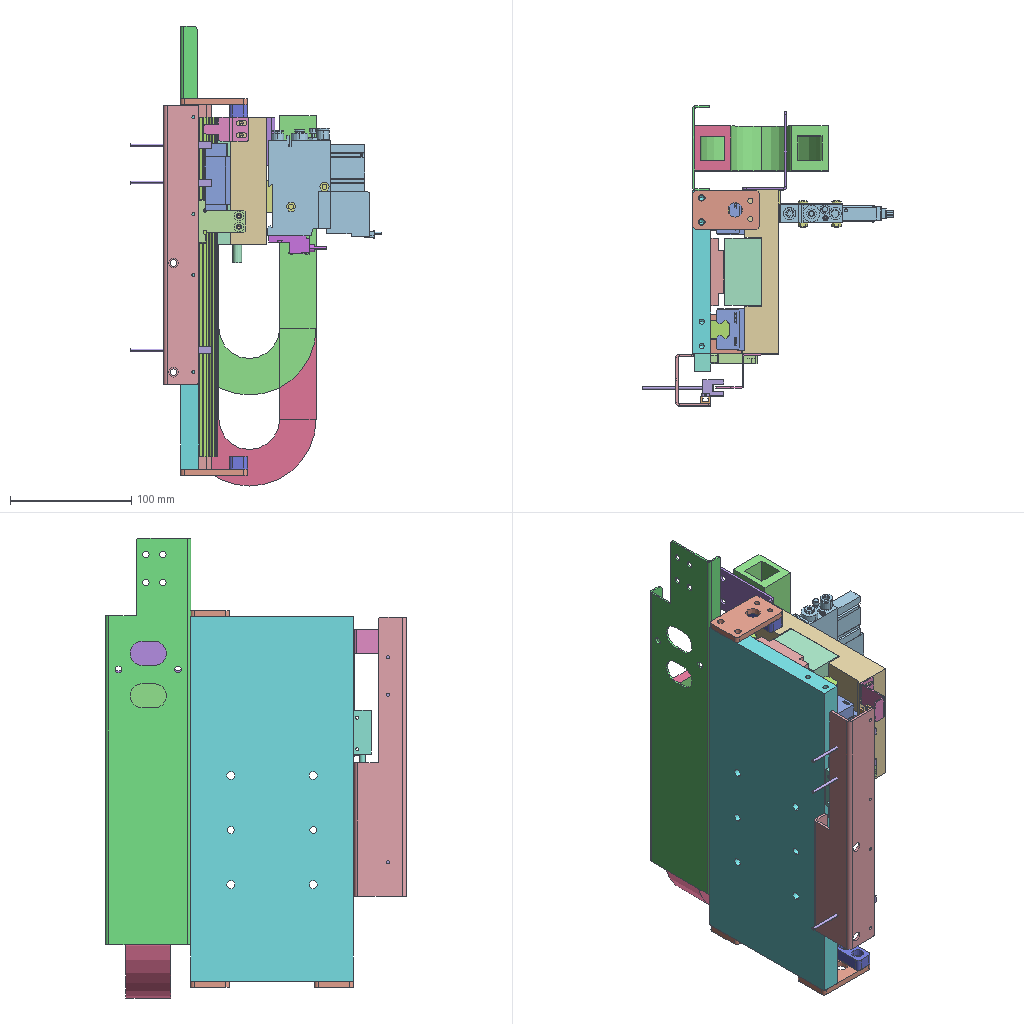Assembly | SolidWorks | 21 different items | 31 placed | box 207 x 248 x 379 mm
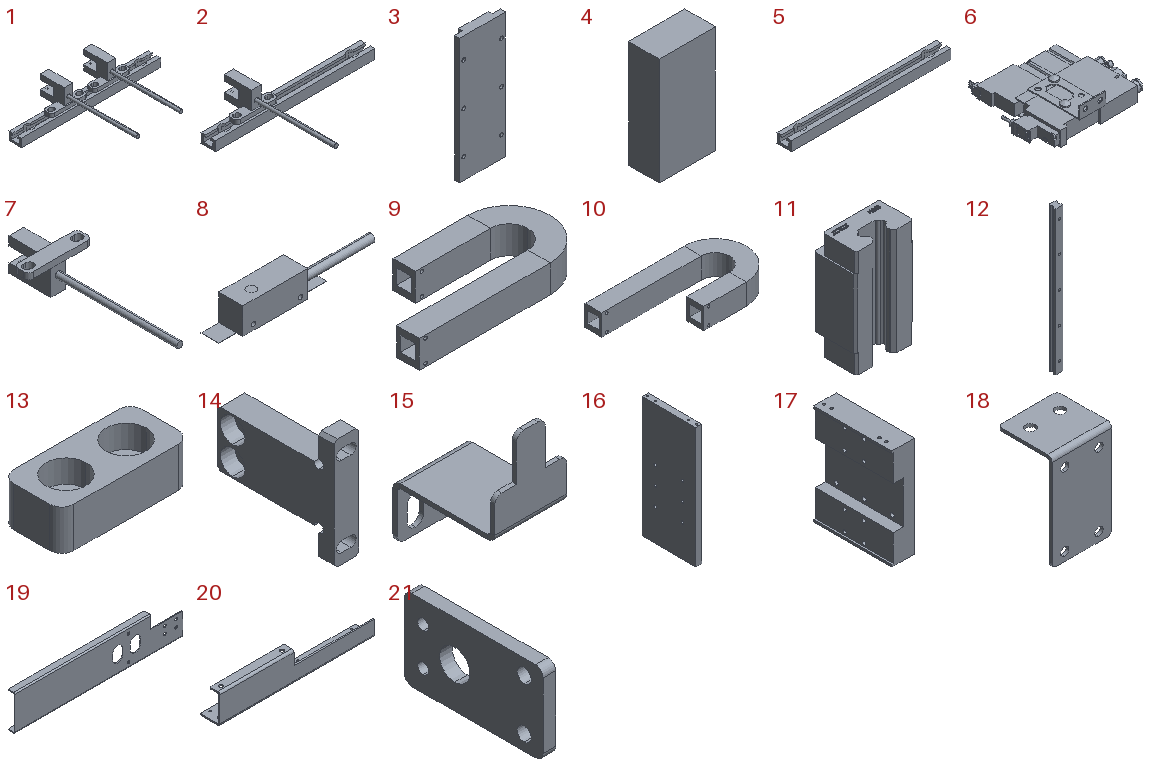Parts list (item | name | quantity | parent item | size | volume | features):
1 | (subassembly) | x1 | - | 100 x 67.2 x 19.7 mm | 6293 mm3 | -
2 | (subassembly) | x1 | - | 100 x 67.2 x 19.7 mm | 4708 mm3 | -
3 | - | x2 | - | 55 x 10.7 x 150 mm | 73163 mm3 | features BaseBody 1
4 | - | x1 | - | 55 x 30 x 120 mm | 172847 mm3 | features BaseBody 1
5 | - | x2 | in 1, 2 | 100 x 9 x 6 mm | 3122 mm3 | features BaseBody 1
6 | - | x1 | - | 104.2 x 94.7 x 31 mm | 87766 mm3 | features BaseBody 3
7 | - | x3 | in 1, 2 | 26 x 67.2 x 13.7 mm | 1586 mm3 | features BaseBody 1
8 | - | x1 | - | 86 x 13.4 x 14.9 mm | 7701 mm3 | features BaseBody 2
9 | - | x1 | - | 230 x 110 x 37 mm | 282563 mm3 | features HoleWzd 2, Sweep 1
10 | - | x1 | - | 230 x 110 x 37 mm | 264813 mm3 | features HoleWzd 2, Sweep 1
11 | - | x2 | - | 34 x 23.7 x 61.7 mm | 37046 mm3 | features BaseBody 1
12 | - | x2 | - | 15 x 15 x 280 mm | 51468 mm3 | features Extrusion 1, HoleWzd 1, ICE 1, LPattern 1
13 | - | x3 | - | 32 x 15 x 10 mm | 3623 mm3 | features Extrusion 1, Fillet 1, HoleWzd 1
14 | - | x1 | - | 8 x 38 x 36 mm | 5326 mm3 | features HoleWzd 2, Chamfer 1, Extrusion 1, ICE 1
15 | - | x1 | - | 20 x 28.2 x 37 mm | 1248 mm3 | features Cut 1, Fillet 1, FlatPattern 1, HoleWzd 1, SMBaseFlange 1, SheetMetal 1
16 | - | x1 | - | 15 x 134 x 300 mm | 594206 mm3 | features HoleWzd 7, Extrusion 1, MirrorPattern 1
17 | - | x1 | - | 30 x 105 x 135 mm | 301604 mm3 | features HoleWzd 9, ICE 2, Extrusion 1, MirrorPattern 1
18 | - | x1 | - | 40 x 36.5 x 65 mm | 7549 mm3 | features HoleWzd 2, Fillet 1, FlatPattern 1, SMBaseFlange 1, SheetMetal 1
19 | - | x1 | - | 335 x 13.5 x 70 mm | 41123 mm3 | features HoleWzd 3, Cut 1, Fillet 1, FlatPattern 1, ICE 1, LPattern 1, SMBaseFlange 1, SheetMetal 1
20 | - | x1 | - | 230 x 29 x 43 mm | 29332 mm3 | features HoleWzd 2, Cut 1, Fillet 1, FlatPattern 1, SMBaseFlange 1, SheetMetal 1
21 | - | x3 | - | 5 x 55 x 32 mm | 7820 mm3 | features HoleWzd 2, Cut 1, Fillet 1, FlatPattern 1, SMBaseFlange 1, SheetMetal 1
Mates (type | each side: item.copy, entity, surface, feature):
In the top assembly
Coincident | 16.1 face plane Boss-Extrude1 | 12.1 face plane Boss-Extrude1
DistanceDim | 12.1 face plane Boss-Extrude1 | 16.1 face plane Boss-Extrude1
Width | 16.1 face plane Boss-Extrude1 | 16.1 face plane Boss-Extrude1 | 12.1 face plane Boss-Extrude1 | 12.1 face plane Boss-Extrude1
Coincident | 16.1 face plane Boss-Extrude1 | 12.2 face plane Boss-Extrude1
Coincident | 12.1 face plane Boss-Extrude1 | 12.2 face plane Boss-Extrude1
Width | 11.1 face plane Input1 | 11.1 face plane Input1 | 12.2 face plane Boss-Extrude1 | 12.2 face plane Boss-Extrude1
Coincident | 12.2 face plane Boss-Extrude1 | 11.1 face plane Input1
Width | 11.2 face plane Input1 | 11.2 face plane Input1 | 12.1 face plane Boss-Extrude1 | 12.1 face plane Boss-Extrude1
Coincident | 12.1 face plane Boss-Extrude1 | 11.2 face plane Input1
Coincident | 11.1 face plane Input1 | 11.2 face plane Input1
Coincident | 11.1 face plane Input1 | 17.1 face plane Cut-Extrude2 | 2 times
Width | 17.1 face plane Boss-Extrude1 | 17.1 face plane Boss-Extrude1 | 11.2 face plane Input1 | 11.2 face plane Input1
Coincident | 17.1 face plane Cut-Extrude1 | 4.1 face plane Input1
Width | 4.1 face plane Input1 | 4.1 face plane Input1 | 17.1 face plane Cut-Extrude1 | 17.1 face plane Cut-Extrude1
Width | 4.1 face plane Input1 | 4.1 face plane Input1 | 17.1 face plane Boss-Extrude1 | 17.1 face plane Boss-Extrude1
LimitDistanceDim | 12.2 face plane Boss-Extrude1 | 17.1 face plane Boss-Extrude1
Coincident | 11.2 face plane Input1 | 17.1 face plane Cut-Extrude2
Coincident | 16.1 face plane Boss-Extrude1 | 3.1 face plane Input1
Width | 16.1 face plane Boss-Extrude1 | 16.1 face plane Boss-Extrude1 | 3.1 face plane Input1 | 3.1 face plane Input1
Coincident | 3.1 face plane Input1 | 3.2 face plane Input1 | 3 times
Width | 16.1 face plane Boss-Extrude1 | 16.1 face plane Boss-Extrude1 | 3.1 face plane Input1 | 3.2 face plane Input1
Coincident | 16.1 face plane Boss-Extrude1 | 21.1 face plane Base-Flange1 | 2 times
Width | 16.1 face plane Boss-Extrude1 | 16.1 face plane Boss-Extrude1 | 21.1 face cylinder M5 Clearance Hole1
Coincident | 16.1 face plane Boss-Extrude1 | 21.2 face plane Base-Flange1 | 2 times
Width | 16.1 face plane Boss-Extrude1 | 16.1 face plane Boss-Extrude1 | 21.2 face cylinder M5 Clearance Hole1
Coincident | 21.2 face plane Base-Flange1 | 13.1 face plane Boss-Extrude1
Coincident | 17.1 face plane Boss-Extrude1 | 14.1 face plane Boss-Extrude1
DistanceDim | 17.1 face plane Boss-Extrude1 | 14.1 face plane Boss-Extrude1 | 2 times
Coincident | 16.1 face plane Boss-Extrude1 | 8.1 face plane Input1 | 2 times
Width | 14.1 face plane M3 Clearance Slot1 | 14.1 face plane M3 Clearance Slot1 | 8.1 face cylinder Input2
Coincident | 17.1 face plane Boss-Extrude1 | 15.1 face plane Base-Flange1 | 3 times
Coincident | 17.1 face plane Boss-Extrude1 | 18.1 face plane Base-Flange1 | 3 times
Coincident | 16.1 face plane Boss-Extrude1 | 19.1 face plane Base-Flange1 | 2 times
DistanceDim | 16.1 face plane Boss-Extrude1 | 19.1 face plane Base-Flange1
Coincident | 10.1 face plane Sweep1 | 19.1 face plane Base-Flange1
Width | 19.1 face plane Base-Flange1 | 19.1 face plane Base-Flange1 | 10.1 face plane Sweep1 | 10.1 face plane Sweep1
Coincident | 17.1 face plane Boss-Extrude1 | 6.1 face plane _ZK2-BK1-A_ZK2_A-1-solid1 | 2 times
DistanceDim | 6.1 face plane _ZK2-BK1-A_ZK2_A-1-solid1 | 17.1 face plane Boss-Extrude1
Coincident | 21.2 face plane Base-Flange1 | 13.2 face plane Boss-Extrude1
Coincident | 21.1 face plane Base-Flange1 | 13.3 face plane Boss-Extrude1
Coincident | 19.1 face plane Base-Flange1 | 9.1 face plane Sweep1
Coincident | 10.1 face plane Sweep1 | 9.1 face plane Sweep1 | 2 times
Concentric | 16.1 face cylinder M5 Tapped Hole1 | 21.3 face cylinder M5 Clearance Hole1 | 2 times
Coincident | 16.1 face plane Boss-Extrude1 | 21.3 face plane Base-Flange1
Coincident | 20.1 face plane Base-Flange1 | 5.1 face plane Input1 | 3 times
Coincident | 20.1 face plane Base-Flange1 | 5.2 face plane Input1 | 3 times
Concentric | 21.2 face cylinder M5 Tapped Hole1 | 13.1 face cylinder CBORE for M5 Hexagon socket head cap screws1 | 2 times
Concentric | 13.2 face cylinder CBORE for M5 Hexagon socket head cap screws1 | 21.3 face cylinder M5 Tapped Hole1 | 2 times
Concentric | 21.1 face cylinder M5 Tapped Hole1 | 13.3 face cylinder CBORE for M5 Hexagon socket head cap screws1 | 2 times
DistanceDim | 10.1 face plane Sweep1 | 19.1 face plane Cut-Extrude1
DistanceDim | 20.1 face plane Base-Flange1 | 16.1 face plane Boss-Extrude1 | 2 times
DistanceDim | 16.1 face plane Boss-Extrude1 | 20.1 face plane Base-Flange1
In subassembly 1
Coincident | 5.3 face plane Input1 | 7.1 face plane Input1
Width | 7.1 face plane Input1 | 7.1 face plane Input1 | 5.3 face plane Input1 | 5.3 face plane Input1
DistanceDim | 7.1 face plane Input1 | 5.3 face plane Input1
Coincident | 5.3 face plane Input1 | 7.2 face plane Input1
Width | 7.2 face plane Input1 | 7.2 face plane Input1 | 5.3 face plane Input1 | 5.3 face plane Input1
DistanceDim | 7.1 face plane Input1 | 7.2 face plane Input1
In subassembly 2
Coincident | 5.3 face plane Input1 | 7.1 face plane Input1
Width | 7.1 face plane Input1 | 7.1 face plane Input1 | 5.3 face plane Input1 | 5.3 face plane Input1
DistanceDim | 7.1 face plane Input1 | 5.3 face plane Input1